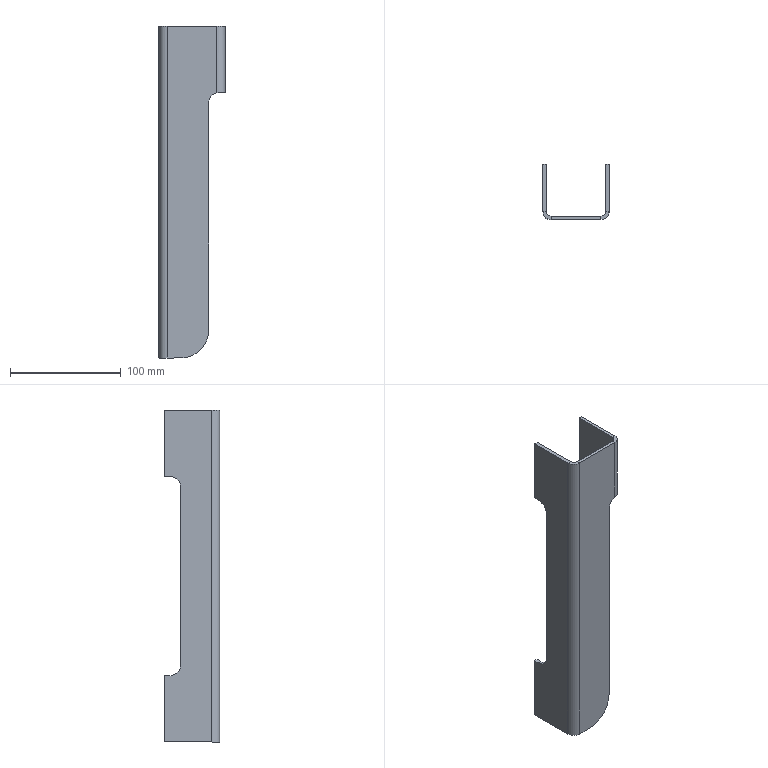Part | SolidWorks | features ICE 2, Fillet 1, FlatPattern 1, SMBaseFlange 1, SheetMetal 1, UnFold 1 | 1 solid | 31 faces | box 60 x 50 x 300 mm | volume 82869 mm3 | plane 22 | cylinder 8 | spline 1 | commonest cylinder face diameters 20 x3 9 x2 15 x2 50 x1
STEP:
#1=CARTESIAN_POINT('',(20.,3.,-150.));
#2=VERTEX_POINT('',#1);
#3=CARTESIAN_POINT('',(7.5,3.,-150.));
#4=VERTEX_POINT('',#3);
#5=CARTESIAN_POINT('',(0.,3.,-150.));
#6=DIRECTION('',(-1.,0.,0.));
#7=VECTOR('',#6,1000.);
#8=LINE('',#5,#7);
#9=EDGE_CURVE('',#2,#4,#8,.T.);
#10=ORIENTED_EDGE('',*,*,#9,.F.);
#11=CARTESIAN_POINT('',(20.,0.,-150.));
#12=VERTEX_POINT('',#11);
#13=CARTESIAN_POINT('',(20.,7.5,-150.));
#14=DIRECTION('',(0.,-1.,0.));
#15=VECTOR('',#14,1000.);
#16=LINE('',#13,#15);
#17=EDGE_CURVE('',#2,#12,#16,.T.);
#18=ORIENTED_EDGE('',*,*,#17,.T.);
#19=CARTESIAN_POINT('',(7.5,0.,-150.));
#20=VERTEX_POINT('',#19);
#21=CARTESIAN_POINT('',(0.,0.,-150.));
#22=DIRECTION('',(-1.,0.,0.));
#23=VECTOR('',#22,1000.);
#24=LINE('',#21,#23);
#25=EDGE_CURVE('',#12,#20,#24,.T.);
#26=ORIENTED_EDGE('',*,*,#25,.T.);
#27=CARTESIAN_POINT('',(7.5,0.,-150.));
#28=DIRECTION('',(0.,1.,0.));
#29=VECTOR('',#28,1000.);
#30=LINE('',#27,#29);
#31=EDGE_CURVE('',#20,#4,#30,.T.);
#32=ORIENTED_EDGE('',*,*,#31,.T.);
#33=EDGE_LOOP('',(#10,#18,#26,#32));
#34=FACE_OUTER_BOUND('',#33,.T.);
#35=CARTESIAN_POINT('',(3.,7.5,-150.));
#36=DIRECTION('',(0.,0.,-1.));
#37=DIRECTION('',(-1.,0.,0.));
#38=AXIS2_PLACEMENT_3D('',#35,#36,#37);
#39=PLANE('',#38);
#40=ADVANCED_FACE('',(#34),#39,.T.);
#41=ORIENTED_EDGE('',*,*,#25,.F.);
#42=CARTESIAN_POINT('',(45.,0.,-125.));
#43=VERTEX_POINT('',#42);
#44=CARTESIAN_POINT('',(20.,0.,-125.));
#45=DIRECTION('',(0.,-1.,0.));
#46=DIRECTION('',(0.,0.,-1.));
#47=AXIS2_PLACEMENT_3D('',#44,#45,#46);
#48=CIRCLE('',#47,25.);
#49=EDGE_CURVE('',#12,#43,#48,.T.);
#50=ORIENTED_EDGE('',*,*,#49,.T.);
#51=CARTESIAN_POINT('',(45.,0.,80.));
#52=VERTEX_POINT('',#51);
#53=CARTESIAN_POINT('',(45.,0.,150.));
#54=DIRECTION('',(0.,0.,-1.));
#55=VECTOR('',#54,1000.);
#56=LINE('',#53,#55);
#57=EDGE_CURVE('',#52,#43,#56,.T.);
#58=ORIENTED_EDGE('',*,*,#57,.F.);
#59=CARTESIAN_POINT('',(52.5,0.,89.682));
#60=VERTEX_POINT('',#59);
#61=CARTESIAN_POINT('',(55.,0.,80.));
#62=DIRECTION('',(0.,-1.,0.));
#63=DIRECTION('',(0.,0.,-1.));
#64=AXIS2_PLACEMENT_3D('',#61,#62,#63);
#65=CIRCLE('',#64,10.);
#66=EDGE_CURVE('',#60,#52,#65,.T.);
#67=ORIENTED_EDGE('',*,*,#66,.F.);
#68=CARTESIAN_POINT('',(52.5,0.,150.));
#69=VERTEX_POINT('',#68);
#70=CARTESIAN_POINT('',(52.5,0.,150.));
#71=DIRECTION('',(0.,0.,-1.));
#72=VECTOR('',#71,1000.);
#73=LINE('',#70,#72);
#74=EDGE_CURVE('',#69,#60,#73,.T.);
#75=ORIENTED_EDGE('',*,*,#74,.F.);
#76=CARTESIAN_POINT('',(7.5,0.,150.));
#77=VERTEX_POINT('',#76);
#78=CARTESIAN_POINT('',(0.,0.,150.));
#79=DIRECTION('',(-1.,0.,0.));
#80=VECTOR('',#79,1000.);
#81=LINE('',#78,#80);
#82=EDGE_CURVE('',#69,#77,#81,.T.);
#83=ORIENTED_EDGE('',*,*,#82,.T.);
#84=CARTESIAN_POINT('',(7.5,0.,150.));
#85=DIRECTION('',(0.,0.,-1.));
#86=VECTOR('',#85,1000.);
#87=LINE('',#84,#86);
#88=EDGE_CURVE('',#77,#20,#87,.T.);
#89=ORIENTED_EDGE('',*,*,#88,.T.);
#90=EDGE_LOOP('',(#41,#50,#58,#67,#75,#83,#89));
#91=FACE_OUTER_BOUND('',#90,.T.);
#92=CARTESIAN_POINT('',(0.,0.,150.));
#93=DIRECTION('',(0.,-1.,0.));
#94=DIRECTION('',(0.,0.,-1.));
#95=AXIS2_PLACEMENT_3D('',#92,#93,#94);
#96=PLANE('',#95);
#97=ADVANCED_FACE('',(#91),#96,.T.);
#98=CARTESIAN_POINT('',(55.,0.4289,90.));
#99=VERTEX_POINT('',#98);
#100=CARTESIAN_POINT('',(52.5,0.,89.682));
#101=CARTESIAN_POINT('',(52.92,0.,89.77));
#102=CARTESIAN_POINT('',(53.343,0.03539,89.841));
#103=CARTESIAN_POINT('',(54.183,0.1789,89.947));
#104=CARTESIAN_POINT('',(54.596,0.2859,89.982));
#105=CARTESIAN_POINT('',(55.,0.4289,90.));
#106=B_SPLINE_CURVE_WITH_KNOTS('',3,(#100,#101,#102,#103,#104,#105),.UNSPECIFIED.,.F.,.F.,(4,2,4),(0.,0.001287,0.002573),.UNSPECIFIED.);
#107=EDGE_CURVE('',#60,#99,#106,.T.);
#108=ORIENTED_EDGE('',*,*,#107,.T.);
#109=CARTESIAN_POINT('',(60.,7.5,90.));
#110=VERTEX_POINT('',#109);
#111=CARTESIAN_POINT('',(52.5,7.5,90.));
#112=DIRECTION('',(0.,0.,1.));
#113=DIRECTION('',(1.,0.,0.));
#114=AXIS2_PLACEMENT_3D('',#111,#112,#113);
#115=CIRCLE('',#114,7.5);
#116=EDGE_CURVE('',#99,#110,#115,.T.);
#117=ORIENTED_EDGE('',*,*,#116,.T.);
#118=CARTESIAN_POINT('',(60.,7.5,150.));
#119=VERTEX_POINT('',#118);
#120=CARTESIAN_POINT('',(60.,7.5,150.));
#121=DIRECTION('',(0.,0.,-1.));
#122=VECTOR('',#121,1000.);
#123=LINE('',#120,#122);
#124=EDGE_CURVE('',#119,#110,#123,.T.);
#125=ORIENTED_EDGE('',*,*,#124,.F.);
#126=CARTESIAN_POINT('',(52.5,7.5,150.));
#127=DIRECTION('',(0.,0.,-1.));
#128=DIRECTION('',(1.,0.,0.));
#129=AXIS2_PLACEMENT_3D('',#126,#127,#128);
#130=CIRCLE('',#129,7.5);
#131=EDGE_CURVE('',#119,#69,#130,.T.);
#132=ORIENTED_EDGE('',*,*,#131,.T.);
#133=ORIENTED_EDGE('',*,*,#74,.T.);
#134=EDGE_LOOP('',(#108,#117,#125,#132,#133));
#135=FACE_OUTER_BOUND('',#134,.T.);
#136=CARTESIAN_POINT('',(52.5,7.5,150.));
#137=DIRECTION('',(0.,0.,-1.));
#138=DIRECTION('',(-1.,0.,0.));
#139=AXIS2_PLACEMENT_3D('',#136,#137,#138);
#140=CYLINDRICAL_SURFACE('',#139,7.5);
#141=ADVANCED_FACE('',(#135),#140,.T.);
#142=ORIENTED_EDGE('',*,*,#124,.T.);
#143=CARTESIAN_POINT('',(60.,50.,90.));
#144=VERTEX_POINT('',#143);
#145=CARTESIAN_POINT('',(60.,50.,90.));
#146=DIRECTION('',(0.,-1.,0.));
#147=VECTOR('',#146,1000.);
#148=LINE('',#145,#147);
#149=EDGE_CURVE('',#144,#110,#148,.T.);
#150=ORIENTED_EDGE('',*,*,#149,.F.);
#151=CARTESIAN_POINT('',(60.,50.,150.));
#152=VERTEX_POINT('',#151);
#153=CARTESIAN_POINT('',(60.,50.,150.));
#154=DIRECTION('',(0.,0.,-1.));
#155=VECTOR('',#154,1000.);
#156=LINE('',#153,#155);
#157=EDGE_CURVE('',#152,#144,#156,.T.);
#158=ORIENTED_EDGE('',*,*,#157,.F.);
#159=CARTESIAN_POINT('',(60.,0.,150.));
#160=DIRECTION('',(0.,-1.,0.));
#161=VECTOR('',#160,1000.);
#162=LINE('',#159,#161);
#163=EDGE_CURVE('',#152,#119,#162,.T.);
#164=ORIENTED_EDGE('',*,*,#163,.T.);
#165=EDGE_LOOP('',(#142,#150,#158,#164));
#166=FACE_OUTER_BOUND('',#165,.T.);
#167=CARTESIAN_POINT('',(60.,0.,150.));
#168=DIRECTION('',(1.,0.,0.));
#169=DIRECTION('',(0.,0.,-1.));
#170=AXIS2_PLACEMENT_3D('',#167,#168,#169);
#171=PLANE('',#170);
#172=ADVANCED_FACE('',(#166),#171,.T.);
#173=CARTESIAN_POINT('',(57.,50.,90.));
#174=VERTEX_POINT('',#173);
#175=CARTESIAN_POINT('',(57.,7.5,90.));
#176=VERTEX_POINT('',#175);
#177=CARTESIAN_POINT('',(57.,0.,90.));
#178=DIRECTION('',(0.,-1.,0.));
#179=VECTOR('',#178,1000.);
#180=LINE('',#177,#179);
#181=EDGE_CURVE('',#174,#176,#180,.T.);
#182=ORIENTED_EDGE('',*,*,#181,.T.);
#183=CARTESIAN_POINT('',(57.,7.5,150.));
#184=VERTEX_POINT('',#183);
#185=CARTESIAN_POINT('',(57.,7.5,150.));
#186=DIRECTION('',(0.,0.,-1.));
#187=VECTOR('',#186,1000.);
#188=LINE('',#185,#187);
#189=EDGE_CURVE('',#184,#176,#188,.T.);
#190=ORIENTED_EDGE('',*,*,#189,.F.);
#191=CARTESIAN_POINT('',(57.,50.,150.));
#192=VERTEX_POINT('',#191);
#193=CARTESIAN_POINT('',(57.,0.,150.));
#194=DIRECTION('',(0.,-1.,0.));
#195=VECTOR('',#194,1000.);
#196=LINE('',#193,#195);
#197=EDGE_CURVE('',#192,#184,#196,.T.);
#198=ORIENTED_EDGE('',*,*,#197,.F.);
#199=CARTESIAN_POINT('',(57.,50.,150.));
#200=DIRECTION('',(0.,0.,-1.));
#201=VECTOR('',#200,1000.);
#202=LINE('',#199,#201);
#203=EDGE_CURVE('',#192,#174,#202,.T.);
#204=ORIENTED_EDGE('',*,*,#203,.T.);
#205=EDGE_LOOP('',(#182,#190,#198,#204));
#206=FACE_OUTER_BOUND('',#205,.T.);
#207=CARTESIAN_POINT('',(57.,0.,150.));
#208=DIRECTION('',(1.,0.,0.));
#209=DIRECTION('',(0.,0.,-1.));
#210=AXIS2_PLACEMENT_3D('',#207,#208,#209);
#211=PLANE('',#210);
#212=ADVANCED_FACE('',(#206),#211,.F.);
#213=CARTESIAN_POINT('',(54.,3.257,90.));
#214=VERTEX_POINT('',#213);
#215=CARTESIAN_POINT('',(52.5,7.5,90.));
#216=DIRECTION('',(0.,0.,1.));
#217=DIRECTION('',(1.,0.,0.));
#218=AXIS2_PLACEMENT_3D('',#215,#216,#217);
#219=CIRCLE('',#218,4.5);
#220=EDGE_CURVE('',#214,#176,#219,.T.);
#221=ORIENTED_EDGE('',*,*,#220,.F.);
#222=CARTESIAN_POINT('',(52.5,3.,89.682));
#223=VERTEX_POINT('',#222);
#224=CARTESIAN_POINT('',(52.5,3.,89.682));
#225=CARTESIAN_POINT('',(52.994,3.,89.855));
#226=CARTESIAN_POINT('',(53.508,3.083,89.964));
#227=CARTESIAN_POINT('',(54.,3.257,90.));
#228=B_SPLINE_CURVE_WITH_KNOTS('',3,(#224,#225,#226,#227),.UNSPECIFIED.,.F.,.F.,(4,4),(0.,0.001563),.UNSPECIFIED.);
#229=EDGE_CURVE('',#223,#214,#228,.T.);
#230=ORIENTED_EDGE('',*,*,#229,.F.);
#231=CARTESIAN_POINT('',(52.5,3.,150.));
#232=VERTEX_POINT('',#231);
#233=CARTESIAN_POINT('',(52.5,3.,150.));
#234=DIRECTION('',(0.,0.,-1.));
#235=VECTOR('',#234,1000.);
#236=LINE('',#233,#235);
#237=EDGE_CURVE('',#232,#223,#236,.T.);
#238=ORIENTED_EDGE('',*,*,#237,.F.);
#239=CARTESIAN_POINT('',(52.5,7.5,150.));
#240=DIRECTION('',(0.,0.,-1.));
#241=DIRECTION('',(1.,0.,0.));
#242=AXIS2_PLACEMENT_3D('',#239,#240,#241);
#243=CIRCLE('',#242,4.5);
#244=EDGE_CURVE('',#184,#232,#243,.T.);
#245=ORIENTED_EDGE('',*,*,#244,.F.);
#246=ORIENTED_EDGE('',*,*,#189,.T.);
#247=EDGE_LOOP('',(#221,#230,#238,#245,#246));
#248=FACE_OUTER_BOUND('',#247,.T.);
#249=CARTESIAN_POINT('',(52.5,7.5,150.));
#250=DIRECTION('',(0.,0.,-1.));
#251=DIRECTION('',(-1.,0.,0.));
#252=AXIS2_PLACEMENT_3D('',#249,#250,#251);
#253=CYLINDRICAL_SURFACE('',#252,4.5);
#254=ADVANCED_FACE('',(#248),#253,.F.);
#255=CARTESIAN_POINT('',(45.,3.,80.));
#256=VERTEX_POINT('',#255);
#257=CARTESIAN_POINT('',(45.,3.,-125.));
#258=VERTEX_POINT('',#257);
#259=CARTESIAN_POINT('',(45.,3.,150.));
#260=DIRECTION('',(0.,0.,-1.));
#261=VECTOR('',#260,1000.);
#262=LINE('',#259,#261);
#263=EDGE_CURVE('',#256,#258,#262,.T.);
#264=ORIENTED_EDGE('',*,*,#263,.T.);
#265=CARTESIAN_POINT('',(20.,3.,-125.));
#266=DIRECTION('',(0.,1.,0.));
#267=DIRECTION('',(0.,0.,-1.));
#268=AXIS2_PLACEMENT_3D('',#265,#266,#267);
#269=CIRCLE('',#268,25.);
#270=EDGE_CURVE('',#258,#2,#269,.T.);
#271=ORIENTED_EDGE('',*,*,#270,.T.);
#272=ORIENTED_EDGE('',*,*,#9,.T.);
#273=CARTESIAN_POINT('',(7.5,3.,150.));
#274=VERTEX_POINT('',#273);
#275=CARTESIAN_POINT('',(7.5,3.,150.));
#276=DIRECTION('',(0.,0.,-1.));
#277=VECTOR('',#276,1000.);
#278=LINE('',#275,#277);
#279=EDGE_CURVE('',#274,#4,#278,.T.);
#280=ORIENTED_EDGE('',*,*,#279,.F.);
#281=CARTESIAN_POINT('',(0.,3.,150.));
#282=DIRECTION('',(-1.,0.,0.));
#283=VECTOR('',#282,1000.);
#284=LINE('',#281,#283);
#285=EDGE_CURVE('',#232,#274,#284,.T.);
#286=ORIENTED_EDGE('',*,*,#285,.F.);
#287=ORIENTED_EDGE('',*,*,#237,.T.);
#288=CARTESIAN_POINT('',(55.,3.,80.));
#289=DIRECTION('',(0.,-1.,0.));
#290=DIRECTION('',(0.,0.,-1.));
#291=AXIS2_PLACEMENT_3D('',#288,#289,#290);
#292=CIRCLE('',#291,10.);
#293=EDGE_CURVE('',#223,#256,#292,.T.);
#294=ORIENTED_EDGE('',*,*,#293,.T.);
#295=EDGE_LOOP('',(#264,#271,#272,#280,#286,#287,#294));
#296=FACE_OUTER_BOUND('',#295,.T.);
#297=CARTESIAN_POINT('',(0.,3.,150.));
#298=DIRECTION('',(0.,-1.,0.));
#299=DIRECTION('',(0.,0.,-1.));
#300=AXIS2_PLACEMENT_3D('',#297,#298,#299);
#301=PLANE('',#300);
#302=ADVANCED_FACE('',(#296),#301,.F.);
#303=CARTESIAN_POINT('',(0.,50.,-90.));
#304=VERTEX_POINT('',#303);
#305=CARTESIAN_POINT('',(3.,50.,-90.));
#306=VERTEX_POINT('',#305);
#307=CARTESIAN_POINT('',(0.,50.,-90.));
#308=DIRECTION('',(1.,0.,0.));
#309=VECTOR('',#308,1000.);
#310=LINE('',#307,#309);
#311=EDGE_CURVE('',#304,#306,#310,.T.);
#312=ORIENTED_EDGE('',*,*,#311,.T.);
#313=CARTESIAN_POINT('',(3.,50.,-150.));
#314=VERTEX_POINT('',#313);
#315=CARTESIAN_POINT('',(3.,50.,150.));
#316=DIRECTION('',(0.,0.,-1.));
#317=VECTOR('',#316,1000.);
#318=LINE('',#315,#317);
#319=EDGE_CURVE('',#306,#314,#318,.T.);
#320=ORIENTED_EDGE('',*,*,#319,.T.);
#321=CARTESIAN_POINT('',(0.,50.,-150.));
#322=VERTEX_POINT('',#321);
#323=CARTESIAN_POINT('',(0.,50.,-150.));
#324=DIRECTION('',(1.,0.,0.));
#325=VECTOR('',#324,1000.);
#326=LINE('',#323,#325);
#327=EDGE_CURVE('',#322,#314,#326,.T.);
#328=ORIENTED_EDGE('',*,*,#327,.F.);
#329=CARTESIAN_POINT('',(0.,50.,150.));
#330=DIRECTION('',(0.,0.,-1.));
#331=VECTOR('',#330,1000.);
#332=LINE('',#329,#331);
#333=EDGE_CURVE('',#304,#322,#332,.T.);
#334=ORIENTED_EDGE('',*,*,#333,.F.);
#335=EDGE_LOOP('',(#312,#320,#328,#334));
#336=FACE_OUTER_BOUND('',#335,.T.);
#337=CARTESIAN_POINT('',(0.,50.,150.));
#338=DIRECTION('',(0.,1.,0.));
#339=DIRECTION('',(0.,0.,1.));
#340=AXIS2_PLACEMENT_3D('',#337,#338,#339);
#341=PLANE('',#340);
#342=ADVANCED_FACE('',(#336),#341,.T.);
#343=CARTESIAN_POINT('',(52.5,0.,150.));
#344=DIRECTION('',(0.,1.,0.));
#345=VECTOR('',#344,1000.);
#346=LINE('',#343,#345);
#347=EDGE_CURVE('',#69,#232,#346,.T.);
#348=ORIENTED_EDGE('',*,*,#347,.F.);
#349=ORIENTED_EDGE('',*,*,#131,.F.);
#350=CARTESIAN_POINT('',(57.,7.5,150.));
#351=DIRECTION('',(1.,0.,0.));
#352=VECTOR('',#351,1000.);
#353=LINE('',#350,#352);
#354=EDGE_CURVE('',#184,#119,#353,.T.);
#355=ORIENTED_EDGE('',*,*,#354,.F.);
#356=ORIENTED_EDGE('',*,*,#244,.T.);
#357=EDGE_LOOP('',(#348,#349,#355,#356));
#358=FACE_OUTER_BOUND('',#357,.T.);
#359=CARTESIAN_POINT('',(52.5,0.,150.));
#360=DIRECTION('',(0.,0.,1.));
#361=DIRECTION('',(1.,0.,0.));
#362=AXIS2_PLACEMENT_3D('',#359,#360,#361);
#363=PLANE('',#362);
#364=ADVANCED_FACE('',(#358),#363,.T.);
#365=ORIENTED_EDGE('',*,*,#82,.F.);
#366=ORIENTED_EDGE('',*,*,#347,.T.);
#367=ORIENTED_EDGE('',*,*,#285,.T.);
#368=CARTESIAN_POINT('',(7.5,3.,150.));
#369=DIRECTION('',(0.,-1.,0.));
#370=VECTOR('',#369,1000.);
#371=LINE('',#368,#370);
#372=EDGE_CURVE('',#274,#77,#371,.T.);
#373=ORIENTED_EDGE('',*,*,#372,.T.);
#374=EDGE_LOOP('',(#365,#366,#367,#373));
#375=FACE_OUTER_BOUND('',#374,.T.);
#376=CARTESIAN_POINT('',(57.,7.5,150.));
#377=DIRECTION('',(0.,0.,1.));
#378=DIRECTION('',(1.,0.,0.));
#379=AXIS2_PLACEMENT_3D('',#376,#377,#378);
#380=PLANE('',#379);
#381=ADVANCED_FACE('',(#375),#380,.T.);
#382=CARTESIAN_POINT('',(0.,7.5,150.));
#383=VERTEX_POINT('',#382);
#384=CARTESIAN_POINT('',(3.,7.5,150.));
#385=VERTEX_POINT('',#384);
#386=CARTESIAN_POINT('',(0.,7.5,150.));
#387=DIRECTION('',(1.,0.,0.));
#388=VECTOR('',#387,1000.);
#389=LINE('',#386,#388);
#390=EDGE_CURVE('',#383,#385,#389,.T.);
#391=ORIENTED_EDGE('',*,*,#390,.F.);
#392=CARTESIAN_POINT('',(7.5,7.5,150.));
#393=DIRECTION('',(0.,0.,-1.));
#394=DIRECTION('',(1.,0.,0.));
#395=AXIS2_PLACEMENT_3D('',#392,#393,#394);
#396=CIRCLE('',#395,7.5);
#397=EDGE_CURVE('',#77,#383,#396,.T.);
#398=ORIENTED_EDGE('',*,*,#397,.F.);
#399=ORIENTED_EDGE('',*,*,#372,.F.);
#400=CARTESIAN_POINT('',(7.5,7.5,150.));
#401=DIRECTION('',(0.,0.,-1.));
#402=DIRECTION('',(1.,0.,0.));
#403=AXIS2_PLACEMENT_3D('',#400,#401,#402);
#404=CIRCLE('',#403,4.5);
#405=EDGE_CURVE('',#274,#385,#404,.T.);
#406=ORIENTED_EDGE('',*,*,#405,.T.);
#407=EDGE_LOOP('',(#391,#398,#399,#406));
#408=FACE_OUTER_BOUND('',#407,.T.);
#409=CARTESIAN_POINT('',(0.,7.5,150.));
#410=DIRECTION('',(0.,0.,1.));
#411=DIRECTION('',(1.,0.,0.));
#412=AXIS2_PLACEMENT_3D('',#409,#410,#411);
#413=PLANE('',#412);
#414=ADVANCED_FACE('',(#408),#413,.T.);
#415=CARTESIAN_POINT('',(0.,50.,150.));
#416=VERTEX_POINT('',#415);
#417=CARTESIAN_POINT('',(0.,0.,150.));
#418=DIRECTION('',(0.,1.,0.));
#419=VECTOR('',#418,1000.);
#420=LINE('',#417,#419);
#421=EDGE_CURVE('',#383,#416,#420,.T.);
#422=ORIENTED_EDGE('',*,*,#421,.F.);
#423=ORIENTED_EDGE('',*,*,#390,.T.);
#424=CARTESIAN_POINT('',(3.,50.,150.));
#425=VERTEX_POINT('',#424);
#426=CARTESIAN_POINT('',(3.,0.,150.));
#427=DIRECTION('',(0.,1.,0.));
#428=VECTOR('',#427,1000.);
#429=LINE('',#426,#428);
#430=EDGE_CURVE('',#385,#425,#429,.T.);
#431=ORIENTED_EDGE('',*,*,#430,.T.);
#432=CARTESIAN_POINT('',(0.,50.,150.));
#433=DIRECTION('',(1.,0.,0.));
#434=VECTOR('',#433,1000.);
#435=LINE('',#432,#434);
#436=EDGE_CURVE('',#416,#425,#435,.T.);
#437=ORIENTED_EDGE('',*,*,#436,.F.);
#438=EDGE_LOOP('',(#422,#423,#431,#437));
#439=FACE_OUTER_BOUND('',#438,.T.);
#440=CARTESIAN_POINT('',(7.5,3.,150.));
#441=DIRECTION('',(0.,0.,1.));
#442=DIRECTION('',(1.,0.,0.));
#443=AXIS2_PLACEMENT_3D('',#440,#441,#442);
#444=PLANE('',#443);
#445=ADVANCED_FACE('',(#439),#444,.T.);
#446=ORIENTED_EDGE('',*,*,#31,.F.);
#447=CARTESIAN_POINT('',(0.,7.5,-150.));
#448=VERTEX_POINT('',#447);
#449=CARTESIAN_POINT('',(7.5,7.5,-150.));
#450=DIRECTION('',(0.,0.,-1.));
#451=DIRECTION('',(1.,0.,0.));
#452=AXIS2_PLACEMENT_3D('',#449,#450,#451);
#453=CIRCLE('',#452,7.5);
#454=EDGE_CURVE('',#20,#448,#453,.T.);
#455=ORIENTED_EDGE('',*,*,#454,.T.);
#456=CARTESIAN_POINT('',(3.,7.5,-150.));
#457=VERTEX_POINT('',#456);
#458=CARTESIAN_POINT('',(3.,7.5,-150.));
#459=DIRECTION('',(-1.,0.,0.));
#460=VECTOR('',#459,1000.);
#461=LINE('',#458,#460);
#462=EDGE_CURVE('',#457,#448,#461,.T.);
#463=ORIENTED_EDGE('',*,*,#462,.F.);
#464=CARTESIAN_POINT('',(7.5,7.5,-150.));
#465=DIRECTION('',(0.,0.,-1.));
#466=DIRECTION('',(1.,0.,0.));
#467=AXIS2_PLACEMENT_3D('',#464,#465,#466);
#468=CIRCLE('',#467,4.5);
#469=EDGE_CURVE('',#4,#457,#468,.T.);
#470=ORIENTED_EDGE('',*,*,#469,.F.);
#471=EDGE_LOOP('',(#446,#455,#463,#470));
#472=FACE_OUTER_BOUND('',#471,.T.);
#473=CARTESIAN_POINT('',(7.5,0.,-150.));
#474=DIRECTION('',(0.,0.,-1.));
#475=DIRECTION('',(-1.,0.,0.));
#476=AXIS2_PLACEMENT_3D('',#473,#474,#475);
#477=PLANE('',#476);
#478=ADVANCED_FACE('',(#472),#477,.T.);
#479=ORIENTED_EDGE('',*,*,#319,.F.);
#480=CARTESIAN_POINT('',(3.,45.,-90.));
#481=VERTEX_POINT('',#480);
#482=CARTESIAN_POINT('',(3.,0.,-90.));
#483=DIRECTION('',(0.,-1.,0.));
#484=VECTOR('',#483,1000.);
#485=LINE('',#482,#484);
#486=EDGE_CURVE('',#306,#481,#485,.T.);
#487=ORIENTED_EDGE('',*,*,#486,.T.);
#488=CARTESIAN_POINT('',(3.,35.,-80.));
#489=VERTEX_POINT('',#488);
#490=CARTESIAN_POINT('',(3.,45.,-80.));
#491=DIRECTION('',(-1.,0.,0.));
#492=DIRECTION('',(0.,0.,1.));
#493=AXIS2_PLACEMENT_3D('',#490,#491,#492);
#494=CIRCLE('',#493,10.);
#495=EDGE_CURVE('',#481,#489,#494,.T.);
#496=ORIENTED_EDGE('',*,*,#495,.T.);
#497=CARTESIAN_POINT('',(3.,35.,80.));
#498=VERTEX_POINT('',#497);
#499=CARTESIAN_POINT('',(3.,35.,150.));
#500=DIRECTION('',(0.,0.,1.));
#501=VECTOR('',#500,1000.);
#502=LINE('',#499,#501);
#503=EDGE_CURVE('',#489,#498,#502,.T.);
#504=ORIENTED_EDGE('',*,*,#503,.T.);
#505=CARTESIAN_POINT('',(3.,45.,90.));
#506=VERTEX_POINT('',#505);
#507=CARTESIAN_POINT('',(3.,45.,80.));
#508=DIRECTION('',(-1.,0.,0.));
#509=DIRECTION('',(0.,0.,1.));
#510=AXIS2_PLACEMENT_3D('',#507,#508,#509);
#511=CIRCLE('',#510,10.);
#512=EDGE_CURVE('',#498,#506,#511,.T.);
#513=ORIENTED_EDGE('',*,*,#512,.T.);
#514=CARTESIAN_POINT('',(3.,50.,90.));
#515=VERTEX_POINT('',#514);
#516=CARTESIAN_POINT('',(3.,0.,90.));
#517=DIRECTION('',(0.,1.,0.));
#518=VECTOR('',#517,1000.);
#519=LINE('',#516,#518);
#520=EDGE_CURVE('',#506,#515,#519,.T.);
#521=ORIENTED_EDGE('',*,*,#520,.T.);
#522=CARTESIAN_POINT('',(3.,50.,150.));
#523=DIRECTION('',(0.,0.,-1.));
#524=VECTOR('',#523,1000.);
#525=LINE('',#522,#524);
#526=EDGE_CURVE('',#425,#515,#525,.T.);
#527=ORIENTED_EDGE('',*,*,#526,.F.);
#528=ORIENTED_EDGE('',*,*,#430,.F.);
#529=CARTESIAN_POINT('',(3.,7.5,150.));
#530=DIRECTION('',(0.,0.,-1.));
#531=VECTOR('',#530,1000.);
#532=LINE('',#529,#531);
#533=EDGE_CURVE('',#385,#457,#532,.T.);
#534=ORIENTED_EDGE('',*,*,#533,.T.);
#535=CARTESIAN_POINT('',(3.,0.,-150.));
#536=DIRECTION('',(0.,1.,0.));
#537=VECTOR('',#536,1000.);
#538=LINE('',#535,#537);
#539=EDGE_CURVE('',#457,#314,#538,.T.);
#540=ORIENTED_EDGE('',*,*,#539,.T.);
#541=EDGE_LOOP('',(#479,#487,#496,#504,#513,#521,#527,#528,#534,#540));
#542=FACE_OUTER_BOUND('',#541,.T.);
#543=CARTESIAN_POINT('',(3.,0.,150.));
#544=DIRECTION('',(-1.,0.,0.));
#545=DIRECTION('',(0.,0.,1.));
#546=AXIS2_PLACEMENT_3D('',#543,#544,#545);
#547=PLANE('',#546);
#548=ADVANCED_FACE('',(#542),#547,.F.);
#549=CARTESIAN_POINT('',(0.,50.,90.));
#550=VERTEX_POINT('',#549);
#551=CARTESIAN_POINT('',(0.,50.,90.));
#552=DIRECTION('',(1.,0.,0.));
#553=VECTOR('',#552,1000.);
#554=LINE('',#551,#553);
#555=EDGE_CURVE('',#550,#515,#554,.T.);
#556=ORIENTED_EDGE('',*,*,#555,.F.);
#557=CARTESIAN_POINT('',(0.,50.,150.));
#558=DIRECTION('',(0.,0.,-1.));
#559=VECTOR('',#558,1000.);
#560=LINE('',#557,#559);
#561=EDGE_CURVE('',#416,#550,#560,.T.);
#562=ORIENTED_EDGE('',*,*,#561,.F.);
#563=ORIENTED_EDGE('',*,*,#436,.T.);
#564=ORIENTED_EDGE('',*,*,#526,.T.);
#565=EDGE_LOOP('',(#556,#562,#563,#564));
#566=FACE_OUTER_BOUND('',#565,.T.);
#567=CARTESIAN_POINT('',(0.,50.,150.));
#568=DIRECTION('',(0.,1.,0.));
#569=DIRECTION('',(0.,0.,1.));
#570=AXIS2_PLACEMENT_3D('',#567,#568,#569);
#571=PLANE('',#570);
#572=ADVANCED_FACE('',(#566),#571,.T.);
#573=CARTESIAN_POINT('',(0.,45.,-90.));
#574=VERTEX_POINT('',#573);
#575=CARTESIAN_POINT('',(0.,45.,-90.));
#576=DIRECTION('',(0.,1.,0.));
#577=VECTOR('',#576,1000.);
#578=LINE('',#575,#577);
#579=EDGE_CURVE('',#574,#304,#578,.T.);
#580=ORIENTED_EDGE('',*,*,#579,.T.);
#581=ORIENTED_EDGE('',*,*,#333,.T.);
#582=CARTESIAN_POINT('',(0.,0.,-150.));
#583=DIRECTION('',(0.,1.,0.));
#584=VECTOR('',#583,1000.);
#585=LINE('',#582,#584);
#586=EDGE_CURVE('',#448,#322,#585,.T.);
#587=ORIENTED_EDGE('',*,*,#586,.F.);
#588=CARTESIAN_POINT('',(0.,7.5,150.));
#589=DIRECTION('',(0.,0.,-1.));
#590=VECTOR('',#589,1000.);
#591=LINE('',#588,#590);
#592=EDGE_CURVE('',#383,#448,#591,.T.);
#593=ORIENTED_EDGE('',*,*,#592,.F.);
#594=ORIENTED_EDGE('',*,*,#421,.T.);
#595=ORIENTED_EDGE('',*,*,#561,.T.);
#596=CARTESIAN_POINT('',(0.,45.,90.));
#597=VERTEX_POINT('',#596);
#598=CARTESIAN_POINT('',(0.,50.,90.));
#599=DIRECTION('',(0.,-1.,0.));
#600=VECTOR('',#599,1000.);
#601=LINE('',#598,#600);
#602=EDGE_CURVE('',#550,#597,#601,.T.);
#603=ORIENTED_EDGE('',*,*,#602,.T.);
#604=CARTESIAN_POINT('',(0.,35.,80.));
#605=VERTEX_POINT('',#604);
#606=CARTESIAN_POINT('',(0.,45.,80.));
#607=DIRECTION('',(1.,0.,0.));
#608=DIRECTION('',(0.,0.,-1.));
#609=AXIS2_PLACEMENT_3D('',#606,#607,#608);
#610=CIRCLE('',#609,10.);
#611=EDGE_CURVE('',#597,#605,#610,.T.);
#612=ORIENTED_EDGE('',*,*,#611,.T.);
#613=CARTESIAN_POINT('',(0.,35.,-80.));
#614=VERTEX_POINT('',#613);
#615=CARTESIAN_POINT('',(0.,35.,80.));
#616=DIRECTION('',(0.,0.,-1.));
#617=VECTOR('',#616,1000.);
#618=LINE('',#615,#617);
#619=EDGE_CURVE('',#605,#614,#618,.T.);
#620=ORIENTED_EDGE('',*,*,#619,.T.);
#621=CARTESIAN_POINT('',(0.,45.,-80.));
#622=DIRECTION('',(1.,0.,0.));
#623=DIRECTION('',(0.,0.,-1.));
#624=AXIS2_PLACEMENT_3D('',#621,#622,#623);
#625=CIRCLE('',#624,10.);
#626=EDGE_CURVE('',#614,#574,#625,.T.);
#627=ORIENTED_EDGE('',*,*,#626,.T.);
#628=EDGE_LOOP('',(#580,#581,#587,#593,#594,#595,#603,#612,#620,#627));
#629=FACE_OUTER_BOUND('',#628,.T.);
#630=CARTESIAN_POINT('',(0.,0.,150.));
#631=DIRECTION('',(-1.,0.,0.));
#632=DIRECTION('',(0.,0.,1.));
#633=AXIS2_PLACEMENT_3D('',#630,#631,#632);
#634=PLANE('',#633);
#635=ADVANCED_FACE('',(#629),#634,.T.);
#636=ORIENTED_EDGE('',*,*,#454,.F.);
#637=ORIENTED_EDGE('',*,*,#88,.F.);
#638=ORIENTED_EDGE('',*,*,#397,.T.);
#639=ORIENTED_EDGE('',*,*,#592,.T.);
#640=EDGE_LOOP('',(#636,#637,#638,#639));
#641=FACE_OUTER_BOUND('',#640,.T.);
#642=CARTESIAN_POINT('',(7.5,7.5,150.));
#643=DIRECTION('',(0.,0.,-1.));
#644=DIRECTION('',(-1.,0.,0.));
#645=AXIS2_PLACEMENT_3D('',#642,#643,#644);
#646=CYLINDRICAL_SURFACE('',#645,7.5);
#647=ADVANCED_FACE('',(#641),#646,.T.);
#648=CARTESIAN_POINT('',(0.,50.,90.));
#649=DIRECTION('',(1.,0.,0.));
#650=VECTOR('',#649,1000.);
#651=LINE('',#648,#650);
#652=EDGE_CURVE('',#174,#144,#651,.T.);
#653=ORIENTED_EDGE('',*,*,#652,.F.);
#654=ORIENTED_EDGE('',*,*,#203,.F.);
#655=CARTESIAN_POINT('',(57.,50.,150.));
#656=DIRECTION('',(1.,0.,0.));
#657=VECTOR('',#656,1000.);
#658=LINE('',#655,#657);
#659=EDGE_CURVE('',#192,#152,#658,.T.);
#660=ORIENTED_EDGE('',*,*,#659,.T.);
#661=ORIENTED_EDGE('',*,*,#157,.T.);
#662=EDGE_LOOP('',(#653,#654,#660,#661));
#663=FACE_OUTER_BOUND('',#662,.T.);
#664=CARTESIAN_POINT('',(57.,50.,150.));
#665=DIRECTION('',(0.,1.,0.));
#666=DIRECTION('',(0.,0.,1.));
#667=AXIS2_PLACEMENT_3D('',#664,#665,#666);
#668=PLANE('',#667);
#669=ADVANCED_FACE('',(#663),#668,.T.);
#670=ORIENTED_EDGE('',*,*,#469,.T.);
#671=ORIENTED_EDGE('',*,*,#533,.F.);
#672=ORIENTED_EDGE('',*,*,#405,.F.);
#673=ORIENTED_EDGE('',*,*,#279,.T.);
#674=EDGE_LOOP('',(#670,#671,#672,#673));
#675=FACE_OUTER_BOUND('',#674,.T.);
#676=CARTESIAN_POINT('',(7.5,7.5,150.));
#677=DIRECTION('',(0.,0.,-1.));
#678=DIRECTION('',(-1.,0.,0.));
#679=AXIS2_PLACEMENT_3D('',#676,#677,#678);
#680=CYLINDRICAL_SURFACE('',#679,4.5);
#681=ADVANCED_FACE('',(#675),#680,.F.);
#682=ORIENTED_EDGE('',*,*,#197,.T.);
#683=ORIENTED_EDGE('',*,*,#354,.T.);
#684=ORIENTED_EDGE('',*,*,#163,.F.);
#685=ORIENTED_EDGE('',*,*,#659,.F.);
#686=EDGE_LOOP('',(#682,#683,#684,#685));
#687=FACE_OUTER_BOUND('',#686,.T.);
#688=CARTESIAN_POINT('',(7.5,7.5,150.));
#689=DIRECTION('',(0.,0.,1.));
#690=DIRECTION('',(1.,0.,0.));
#691=AXIS2_PLACEMENT_3D('',#688,#689,#690);
#692=PLANE('',#691);
#693=ADVANCED_FACE('',(#687),#692,.T.);
#694=ORIENTED_EDGE('',*,*,#539,.F.);
#695=ORIENTED_EDGE('',*,*,#462,.T.);
#696=ORIENTED_EDGE('',*,*,#586,.T.);
#697=ORIENTED_EDGE('',*,*,#327,.T.);
#698=EDGE_LOOP('',(#694,#695,#696,#697));
#699=FACE_OUTER_BOUND('',#698,.T.);
#700=CARTESIAN_POINT('',(7.5,7.5,-150.));
#701=DIRECTION('',(0.,0.,1.));
#702=DIRECTION('',(1.,0.,0.));
#703=AXIS2_PLACEMENT_3D('',#700,#701,#702);
#704=PLANE('',#703);
#705=ADVANCED_FACE('',(#699),#704,.F.);
#706=ORIENTED_EDGE('',*,*,#652,.T.);
#707=ORIENTED_EDGE('',*,*,#149,.T.);
#708=ORIENTED_EDGE('',*,*,#116,.F.);
#709=CARTESIAN_POINT('',(55.,0.4289,90.));
#710=DIRECTION('',(0.3333,-0.9428,0.));
#711=VECTOR('',#710,1000.);
#712=LINE('',#709,#711);
#713=EDGE_CURVE('',#214,#99,#712,.T.);
#714=ORIENTED_EDGE('',*,*,#713,.F.);
#715=ORIENTED_EDGE('',*,*,#220,.T.);
#716=ORIENTED_EDGE('',*,*,#181,.F.);
#717=EDGE_LOOP('',(#706,#707,#708,#714,#715,#716));
#718=FACE_OUTER_BOUND('',#717,.T.);
#719=CARTESIAN_POINT('',(0.,50.,90.));
#720=DIRECTION('',(0.,0.,1.));
#721=DIRECTION('',(1.,0.,0.));
#722=AXIS2_PLACEMENT_3D('',#719,#720,#721);
#723=PLANE('',#722);
#724=ADVANCED_FACE('',(#718),#723,.F.);
#725=ORIENTED_EDGE('',*,*,#311,.F.);
#726=ORIENTED_EDGE('',*,*,#579,.F.);
#727=CARTESIAN_POINT('',(0.,45.,-90.));
#728=DIRECTION('',(1.,0.,0.));
#729=VECTOR('',#728,1000.);
#730=LINE('',#727,#729);
#731=EDGE_CURVE('',#574,#481,#730,.T.);
#732=ORIENTED_EDGE('',*,*,#731,.T.);
#733=ORIENTED_EDGE('',*,*,#486,.F.);
#734=EDGE_LOOP('',(#725,#726,#732,#733));
#735=FACE_OUTER_BOUND('',#734,.T.);
#736=CARTESIAN_POINT('',(0.,45.,-90.));
#737=DIRECTION('',(0.,0.,-1.));
#738=DIRECTION('',(-1.,0.,0.));
#739=AXIS2_PLACEMENT_3D('',#736,#737,#738);
#740=PLANE('',#739);
#741=ADVANCED_FACE('',(#735),#740,.F.);
#742=ORIENTED_EDGE('',*,*,#731,.F.);
#743=ORIENTED_EDGE('',*,*,#626,.F.);
#744=CARTESIAN_POINT('',(0.,35.,-80.));
#745=DIRECTION('',(1.,0.,0.));
#746=VECTOR('',#745,1000.);
#747=LINE('',#744,#746);
#748=EDGE_CURVE('',#614,#489,#747,.T.);
#749=ORIENTED_EDGE('',*,*,#748,.T.);
#750=ORIENTED_EDGE('',*,*,#495,.F.);
#751=EDGE_LOOP('',(#742,#743,#749,#750));
#752=FACE_OUTER_BOUND('',#751,.T.);
#753=CARTESIAN_POINT('',(0.,45.,-80.));
#754=DIRECTION('',(1.,0.,0.));
#755=DIRECTION('',(0.,0.,-1.));
#756=AXIS2_PLACEMENT_3D('',#753,#754,#755);
#757=CYLINDRICAL_SURFACE('',#756,10.);
#758=ADVANCED_FACE('',(#752),#757,.F.);
#759=ORIENTED_EDGE('',*,*,#748,.F.);
#760=ORIENTED_EDGE('',*,*,#619,.F.);
#761=CARTESIAN_POINT('',(0.,35.,80.));
#762=DIRECTION('',(1.,0.,0.));
#763=VECTOR('',#762,1000.);
#764=LINE('',#761,#763);
#765=EDGE_CURVE('',#605,#498,#764,.T.);
#766=ORIENTED_EDGE('',*,*,#765,.T.);
#767=ORIENTED_EDGE('',*,*,#503,.F.);
#768=EDGE_LOOP('',(#759,#760,#766,#767));
#769=FACE_OUTER_BOUND('',#768,.T.);
#770=CARTESIAN_POINT('',(0.,35.,80.));
#771=DIRECTION('',(0.,-1.,0.));
#772=DIRECTION('',(0.,0.,-1.));
#773=AXIS2_PLACEMENT_3D('',#770,#771,#772);
#774=PLANE('',#773);
#775=ADVANCED_FACE('',(#769),#774,.F.);
#776=ORIENTED_EDGE('',*,*,#765,.F.);
#777=ORIENTED_EDGE('',*,*,#611,.F.);
#778=CARTESIAN_POINT('',(0.,45.,90.));
#779=DIRECTION('',(1.,0.,0.));
#780=VECTOR('',#779,1000.);
#781=LINE('',#778,#780);
#782=EDGE_CURVE('',#597,#506,#781,.T.);
#783=ORIENTED_EDGE('',*,*,#782,.T.);
#784=ORIENTED_EDGE('',*,*,#512,.F.);
#785=EDGE_LOOP('',(#776,#777,#783,#784));
#786=FACE_OUTER_BOUND('',#785,.T.);
#787=CARTESIAN_POINT('',(0.,45.,80.));
#788=DIRECTION('',(1.,0.,0.));
#789=DIRECTION('',(0.,0.,-1.));
#790=AXIS2_PLACEMENT_3D('',#787,#788,#789);
#791=CYLINDRICAL_SURFACE('',#790,10.);
#792=ADVANCED_FACE('',(#786),#791,.F.);
#793=ORIENTED_EDGE('',*,*,#782,.F.);
#794=ORIENTED_EDGE('',*,*,#602,.F.);
#795=ORIENTED_EDGE('',*,*,#555,.T.);
#796=ORIENTED_EDGE('',*,*,#520,.F.);
#797=EDGE_LOOP('',(#793,#794,#795,#796));
#798=FACE_OUTER_BOUND('',#797,.T.);
#799=CARTESIAN_POINT('',(0.,50.,90.));
#800=DIRECTION('',(0.,0.,1.));
#801=DIRECTION('',(1.,0.,0.));
#802=AXIS2_PLACEMENT_3D('',#799,#800,#801);
#803=PLANE('',#802);
#804=ADVANCED_FACE('',(#798),#803,.F.);
#805=CARTESIAN_POINT('',(52.5,3.,89.682));
#806=DIRECTION('',(0.,-1.,0.));
#807=VECTOR('',#806,1000.);
#808=LINE('',#805,#807);
#809=EDGE_CURVE('',#223,#60,#808,.T.);
#810=ORIENTED_EDGE('',*,*,#809,.F.);
#811=ORIENTED_EDGE('',*,*,#229,.T.);
#812=ORIENTED_EDGE('',*,*,#713,.T.);
#813=ORIENTED_EDGE('',*,*,#107,.F.);
#814=EDGE_LOOP('',(#810,#811,#812,#813));
#815=FACE_OUTER_BOUND('',#814,.T.);
#816=CARTESIAN_POINT('',(52.5,-0.03,89.682));
#817=CARTESIAN_POINT('',(53.344,-0.03,89.858));
#818=CARTESIAN_POINT('',(54.197,0.1131,89.964));
#819=CARTESIAN_POINT('',(55.01,0.4006,90.));
#820=CARTESIAN_POINT('',(52.5,0.,89.682));
#821=CARTESIAN_POINT('',(53.341,0.,89.858));
#822=CARTESIAN_POINT('',(54.19,0.1425,89.964));
#823=CARTESIAN_POINT('',(55.,0.4289,90.));
#824=CARTESIAN_POINT('',(52.5,3.,89.682));
#825=CARTESIAN_POINT('',(53.004,3.,89.858));
#826=CARTESIAN_POINT('',(53.514,3.086,89.964));
#827=CARTESIAN_POINT('',(54.,3.257,90.));
#828=B_SPLINE_SURFACE_WITH_KNOTS('',1,3,((#816,#817,#818,#819),(#820,#821,#822,#823),(#824,#825,#826,#827)),.UNSPECIFIED.,.F.,.F.,.F.,(2,1,2),(4,4),(-0.01,0.,1.),(0.,1.),.UNSPECIFIED.);
#829=ADVANCED_FACE('',(#815),#828,.T.);
#830=ORIENTED_EDGE('',*,*,#293,.F.);
#831=ORIENTED_EDGE('',*,*,#809,.T.);
#832=ORIENTED_EDGE('',*,*,#66,.T.);
#833=CARTESIAN_POINT('',(45.,3.,80.));
#834=DIRECTION('',(0.,-1.,0.));
#835=VECTOR('',#834,1000.);
#836=LINE('',#833,#835);
#837=EDGE_CURVE('',#256,#52,#836,.T.);
#838=ORIENTED_EDGE('',*,*,#837,.F.);
#839=EDGE_LOOP('',(#830,#831,#832,#838));
#840=FACE_OUTER_BOUND('',#839,.T.);
#841=CARTESIAN_POINT('',(55.,3.,80.));
#842=DIRECTION('',(0.,-1.,0.));
#843=DIRECTION('',(0.,0.,-1.));
#844=AXIS2_PLACEMENT_3D('',#841,#842,#843);
#845=CYLINDRICAL_SURFACE('',#844,10.);
#846=ADVANCED_FACE('',(#840),#845,.F.);
#847=ORIENTED_EDGE('',*,*,#57,.T.);
#848=CARTESIAN_POINT('',(45.,3.,-125.));
#849=DIRECTION('',(0.,1.,0.));
#850=VECTOR('',#849,1000.);
#851=LINE('',#848,#850);
#852=EDGE_CURVE('',#43,#258,#851,.T.);
#853=ORIENTED_EDGE('',*,*,#852,.T.);
#854=ORIENTED_EDGE('',*,*,#263,.F.);
#855=ORIENTED_EDGE('',*,*,#837,.T.);
#856=EDGE_LOOP('',(#847,#853,#854,#855));
#857=FACE_OUTER_BOUND('',#856,.T.);
#858=CARTESIAN_POINT('',(45.,3.,150.));
#859=DIRECTION('',(-1.,0.,0.));
#860=DIRECTION('',(0.,0.,-1.));
#861=AXIS2_PLACEMENT_3D('',#858,#859,#860);
#862=PLANE('',#861);
#863=ADVANCED_FACE('',(#857),#862,.F.);
#864=ORIENTED_EDGE('',*,*,#270,.F.);
#865=ORIENTED_EDGE('',*,*,#852,.F.);
#866=ORIENTED_EDGE('',*,*,#49,.F.);
#867=ORIENTED_EDGE('',*,*,#17,.F.);
#868=EDGE_LOOP('',(#864,#865,#866,#867));
#869=FACE_OUTER_BOUND('',#868,.T.);
#870=CARTESIAN_POINT('',(20.,7.5,-125.));
#871=DIRECTION('',(0.,1.,0.));
#872=DIRECTION('',(0.,0.,1.));
#873=AXIS2_PLACEMENT_3D('',#870,#871,#872);
#874=CYLINDRICAL_SURFACE('',#873,25.);
#875=ADVANCED_FACE('',(#869),#874,.T.);
#876=CLOSED_SHELL('',(#40,#97,#141,#172,#212,#254,#302,#342,#364,#381,#414,#445,#478,#548,#572,#635,#647,#669,#681,#693,#705,#724,#741,#758,#775,#792,#804,#829,#846,#863,#875));
#877=MANIFOLD_SOLID_BREP('',#876);
#878=CARTESIAN_POINT('',(0.,0.,0.));
#879=DIRECTION('',(0.,0.,1.));
#880=DIRECTION('',(1.,0.,0.));
#881=AXIS2_PLACEMENT_3D('',#878,#879,#880);
#882=(LENGTH_UNIT()NAMED_UNIT(*)SI_UNIT(.MILLI.,.METRE.));
#883=UNCERTAINTY_MEASURE_WITH_UNIT(LENGTH_MEASURE(0.00001),#882,'','');
#884=(NAMED_UNIT(*)PLANE_ANGLE_UNIT()SI_UNIT($,.RADIAN.));
#885=(NAMED_UNIT(*)SI_UNIT($,.STERADIAN.)SOLID_ANGLE_UNIT());
#886=(GEOMETRIC_REPRESENTATION_CONTEXT(3)GLOBAL_UNCERTAINTY_ASSIGNED_CONTEXT((#883))GLOBAL_UNIT_ASSIGNED_CONTEXT((#882,#884,#885))REPRESENTATION_CONTEXT('',''));
#887=ADVANCED_BREP_SHAPE_REPRESENTATION('',(#877,#881),#886);